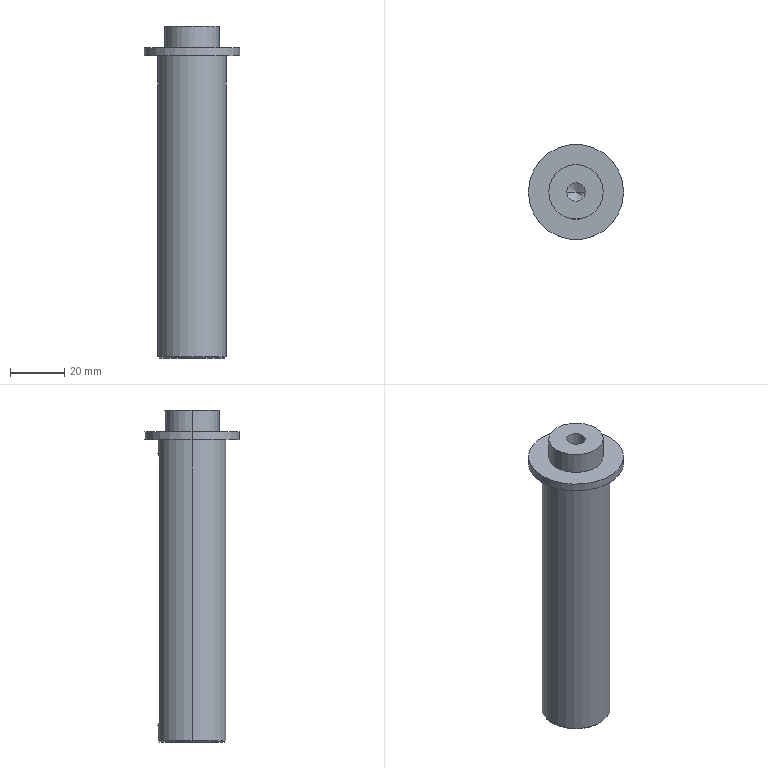Part | SolidWorks | features ICE 3, HoleWzd 2, Chamfer 1, Extrusion 1 | 1 solid | 26 faces | box 35 x 35 x 122 mm | volume 53457 mm3 | cylinder 13 | plane 7 | cone 6 | commonest cylinder face diameters 8 x3 6.8 x2 10.2 x2 20 x2 25 x2 35 x2
STEP:
#1=CARTESIAN_POINT('',(-12.,0.,0.));
#2=VERTEX_POINT('',#1);
#3=CARTESIAN_POINT('',(12.,0.,0.));
#4=VERTEX_POINT('',#3);
#5=CARTESIAN_POINT('',(0.,0.,0.));
#6=DIRECTION('',(0.,0.,-1.));
#7=DIRECTION('',(1.,0.,0.));
#8=AXIS2_PLACEMENT_3D('',#5,#6,#7);
#9=CIRCLE('',#8,12.);
#10=EDGE_CURVE('',#2,#4,#9,.T.);
#11=ORIENTED_EDGE('',*,*,#10,.F.);
#12=CARTESIAN_POINT('',(-12.5,0.,0.5));
#13=VERTEX_POINT('',#12);
#14=CARTESIAN_POINT('',(-12.5,0.,0.5));
#15=DIRECTION('',(-0.7071,0.,0.7071));
#16=VECTOR('',#15,1000.);
#17=LINE('',#14,#16);
#18=EDGE_CURVE('',#2,#13,#17,.T.);
#19=ORIENTED_EDGE('',*,*,#18,.T.);
#20=CARTESIAN_POINT('',(12.5,0.,0.5));
#21=VERTEX_POINT('',#20);
#22=CARTESIAN_POINT('',(0.,0.,0.5));
#23=DIRECTION('',(0.,0.,1.));
#24=DIRECTION('',(1.,0.,0.));
#25=AXIS2_PLACEMENT_3D('',#22,#23,#24);
#26=CIRCLE('',#25,12.5);
#27=EDGE_CURVE('',#21,#13,#26,.T.);
#28=ORIENTED_EDGE('',*,*,#27,.F.);
#29=CARTESIAN_POINT('',(12.5,0.,0.5));
#30=DIRECTION('',(0.7071,0.,0.7071));
#31=VECTOR('',#30,1000.);
#32=LINE('',#29,#31);
#33=EDGE_CURVE('',#4,#21,#32,.T.);
#34=ORIENTED_EDGE('',*,*,#33,.F.);
#35=EDGE_LOOP('',(#11,#19,#28,#34));
#36=FACE_OUTER_BOUND('',#35,.T.);
#37=CARTESIAN_POINT('',(0.,0.,0.5));
#38=DIRECTION('',(0.,0.,1.));
#39=DIRECTION('',(1.,0.,0.));
#40=AXIS2_PLACEMENT_3D('',#37,#38,#39);
#41=CONICAL_SURFACE('',#40,12.5,0.7854);
#42=ADVANCED_FACE('',(#36),#41,.T.);
#43=CARTESIAN_POINT('',(5.1,0.,30.25));
#44=VERTEX_POINT('',#43);
#45=CARTESIAN_POINT('',(-5.1,0.,30.25));
#46=VERTEX_POINT('',#45);
#47=CARTESIAN_POINT('',(0.,0.,30.25));
#48=DIRECTION('',(0.,0.,-1.));
#49=DIRECTION('',(-1.,0.,0.));
#50=AXIS2_PLACEMENT_3D('',#47,#48,#49);
#51=CIRCLE('',#50,5.1);
#52=EDGE_CURVE('',#44,#46,#51,.T.);
#53=ORIENTED_EDGE('',*,*,#52,.F.);
#54=CARTESIAN_POINT('',(5.1,0.,0.));
#55=VERTEX_POINT('',#54);
#56=CARTESIAN_POINT('',(5.1,0.,0.));
#57=DIRECTION('',(0.,0.,-1.));
#58=VECTOR('',#57,1000.);
#59=LINE('',#56,#58);
#60=EDGE_CURVE('',#44,#55,#59,.T.);
#61=ORIENTED_EDGE('',*,*,#60,.T.);
#62=CARTESIAN_POINT('',(-5.1,0.,0.));
#63=VERTEX_POINT('',#62);
#64=CARTESIAN_POINT('',(0.,0.,0.));
#65=DIRECTION('',(0.,0.,-1.));
#66=DIRECTION('',(-1.,0.,0.));
#67=AXIS2_PLACEMENT_3D('',#64,#65,#66);
#68=CIRCLE('',#67,5.1);
#69=EDGE_CURVE('',#55,#63,#68,.T.);
#70=ORIENTED_EDGE('',*,*,#69,.T.);
#71=CARTESIAN_POINT('',(-5.1,0.,0.));
#72=DIRECTION('',(0.,0.,-1.));
#73=VECTOR('',#72,1000.);
#74=LINE('',#71,#73);
#75=EDGE_CURVE('',#46,#63,#74,.T.);
#76=ORIENTED_EDGE('',*,*,#75,.F.);
#77=EDGE_LOOP('',(#53,#61,#70,#76));
#78=FACE_OUTER_BOUND('',#77,.T.);
#79=CARTESIAN_POINT('',(0.,0.,0.));
#80=DIRECTION('',(0.,0.,-1.));
#81=DIRECTION('',(-1.,0.,0.));
#82=AXIS2_PLACEMENT_3D('',#79,#80,#81);
#83=CYLINDRICAL_SURFACE('',#82,5.1);
#84=ADVANCED_FACE('',(#78),#83,.F.);
#85=CARTESIAN_POINT('',(0.,0.,33.314));
#86=VERTEX_POINT('',#85);
#87=CARTESIAN_POINT('',(-5.1,0.,30.25));
#88=DIRECTION('',(-0.8572,0.,-0.515));
#89=VECTOR('',#88,1000.);
#90=LINE('',#87,#89);
#91=EDGE_CURVE('',#86,#46,#90,.T.);
#92=ORIENTED_EDGE('',*,*,#91,.F.);
#93=CARTESIAN_POINT('',(5.1,0.,30.25));
#94=DIRECTION('',(0.8572,0.,-0.515));
#95=VECTOR('',#94,1000.);
#96=LINE('',#93,#95);
#97=EDGE_CURVE('',#86,#44,#96,.T.);
#98=ORIENTED_EDGE('',*,*,#97,.T.);
#99=ORIENTED_EDGE('',*,*,#52,.T.);
#100=EDGE_LOOP('',(#92,#98,#99));
#101=FACE_OUTER_BOUND('',#100,.T.);
#102=CARTESIAN_POINT('',(0.,0.,30.25));
#103=DIRECTION('',(0.,0.,-1.));
#104=DIRECTION('',(-1.,0.,0.));
#105=AXIS2_PLACEMENT_3D('',#102,#103,#104);
#106=CONICAL_SURFACE('',#105,5.1,1.03);
#107=ADVANCED_FACE('',(#101),#106,.F.);
#108=CARTESIAN_POINT('',(-3.4,0.,98.25));
#109=VERTEX_POINT('',#108);
#110=CARTESIAN_POINT('',(3.4,0.,98.25));
#111=VERTEX_POINT('',#110);
#112=CARTESIAN_POINT('',(0.,0.,98.25));
#113=DIRECTION('',(0.,0.,1.));
#114=DIRECTION('',(1.,0.,0.));
#115=AXIS2_PLACEMENT_3D('',#112,#113,#114);
#116=CIRCLE('',#115,3.4);
#117=EDGE_CURVE('',#109,#111,#116,.T.);
#118=ORIENTED_EDGE('',*,*,#117,.F.);
#119=CARTESIAN_POINT('',(-3.4,0.,122.));
#120=VERTEX_POINT('',#119);
#121=CARTESIAN_POINT('',(-3.4,0.,122.));
#122=DIRECTION('',(0.,0.,1.));
#123=VECTOR('',#122,1000.);
#124=LINE('',#121,#123);
#125=EDGE_CURVE('',#109,#120,#124,.T.);
#126=ORIENTED_EDGE('',*,*,#125,.T.);
#127=CARTESIAN_POINT('',(3.4,0.,122.));
#128=VERTEX_POINT('',#127);
#129=CARTESIAN_POINT('',(0.,0.,122.));
#130=DIRECTION('',(0.,0.,1.));
#131=DIRECTION('',(1.,0.,0.));
#132=AXIS2_PLACEMENT_3D('',#129,#130,#131);
#133=CIRCLE('',#132,3.4);
#134=EDGE_CURVE('',#120,#128,#133,.T.);
#135=ORIENTED_EDGE('',*,*,#134,.T.);
#136=CARTESIAN_POINT('',(3.4,0.,122.));
#137=DIRECTION('',(0.,0.,1.));
#138=VECTOR('',#137,1000.);
#139=LINE('',#136,#138);
#140=EDGE_CURVE('',#111,#128,#139,.T.);
#141=ORIENTED_EDGE('',*,*,#140,.F.);
#142=EDGE_LOOP('',(#118,#126,#135,#141));
#143=FACE_OUTER_BOUND('',#142,.T.);
#144=CARTESIAN_POINT('',(0.,0.,122.));
#145=DIRECTION('',(0.,0.,1.));
#146=DIRECTION('',(1.,0.,0.));
#147=AXIS2_PLACEMENT_3D('',#144,#145,#146);
#148=CYLINDRICAL_SURFACE('',#147,3.4);
#149=ADVANCED_FACE('',(#143),#148,.F.);
#150=CARTESIAN_POINT('',(0.,0.,96.207));
#151=VERTEX_POINT('',#150);
#152=CARTESIAN_POINT('',(3.4,0.,98.25));
#153=DIRECTION('',(0.8572,0.,0.515));
#154=VECTOR('',#153,1000.);
#155=LINE('',#152,#154);
#156=EDGE_CURVE('',#151,#111,#155,.T.);
#157=ORIENTED_EDGE('',*,*,#156,.F.);
#158=CARTESIAN_POINT('',(-3.4,0.,98.25));
#159=DIRECTION('',(-0.8572,0.,0.515));
#160=VECTOR('',#159,1000.);
#161=LINE('',#158,#160);
#162=EDGE_CURVE('',#151,#109,#161,.T.);
#163=ORIENTED_EDGE('',*,*,#162,.T.);
#164=ORIENTED_EDGE('',*,*,#117,.T.);
#165=EDGE_LOOP('',(#157,#163,#164));
#166=FACE_OUTER_BOUND('',#165,.T.);
#167=CARTESIAN_POINT('',(0.,0.,98.25));
#168=DIRECTION('',(0.,0.,1.));
#169=DIRECTION('',(1.,0.,0.));
#170=AXIS2_PLACEMENT_3D('',#167,#168,#169);
#171=CONICAL_SURFACE('',#170,3.4,1.03);
#172=ADVANCED_FACE('',(#166),#171,.F.);
#173=CARTESIAN_POINT('',(0.,8.5,106.));
#174=VERTEX_POINT('',#173);
#175=CARTESIAN_POINT('',(4.,8.5,102.));
#176=VERTEX_POINT('',#175);
#177=CARTESIAN_POINT('',(0.,8.5,102.));
#178=DIRECTION('',(0.,1.,0.));
#179=DIRECTION('',(0.,0.,1.));
#180=AXIS2_PLACEMENT_3D('',#177,#178,#179);
#181=CIRCLE('',#180,4.);
#182=EDGE_CURVE('',#174,#176,#181,.T.);
#183=ORIENTED_EDGE('',*,*,#182,.F.);
#184=CARTESIAN_POINT('',(0.,12.5,106.));
#185=VERTEX_POINT('',#184);
#186=CARTESIAN_POINT('',(0.,8.5,106.));
#187=DIRECTION('',(0.,1.,0.));
#188=VECTOR('',#187,1000.);
#189=LINE('',#186,#188);
#190=EDGE_CURVE('',#174,#185,#189,.T.);
#191=ORIENTED_EDGE('',*,*,#190,.T.);
#192=CARTESIAN_POINT('',(4.,11.843,102.));
#193=VERTEX_POINT('',#192);
#194=CARTESIAN_POINT('',(4.,11.843,102.));
#195=CARTESIAN_POINT('',(4.,11.843,102.266));
#196=CARTESIAN_POINT('',(3.974,11.852,102.528));
#197=CARTESIAN_POINT('',(3.871,11.886,103.041));
#198=CARTESIAN_POINT('',(3.793,11.911,103.296));
#199=CARTESIAN_POINT('',(3.592,11.973,103.78));
#200=CARTESIAN_POINT('',(3.469,12.01,104.009));
#201=CARTESIAN_POINT('',(3.178,12.09,104.443));
#202=CARTESIAN_POINT('',(3.011,12.134,104.646));
#203=CARTESIAN_POINT('',(2.644,12.219,105.013));
#204=CARTESIAN_POINT('',(2.444,12.261,105.178));
#205=CARTESIAN_POINT('',(2.006,12.34,105.47));
#206=CARTESIAN_POINT('',(1.776,12.375,105.593));
#207=CARTESIAN_POINT('',(1.295,12.435,105.793));
#208=CARTESIAN_POINT('',(1.041,12.459,105.871));
#209=CARTESIAN_POINT('',(0.5239,12.492,105.974));
#210=CARTESIAN_POINT('',(0.263,12.5,106.));
#211=CARTESIAN_POINT('',(0.,12.5,106.));
#212=B_SPLINE_CURVE_WITH_KNOTS('',3,(#194,#195,#196,#197,#198,#199,#200,#201,#202,#203,#204,#205,#206,#207,#208,#209,#210,#211),.UNSPECIFIED.,.F.,.F.,(4,2,2,2,2,2,2,2,4),(0.,0.000787,0.001574,0.002361,0.003148,0.003935,0.004722,0.005509,0.006296),.UNSPECIFIED.);
#213=EDGE_CURVE('',#193,#185,#212,.T.);
#214=ORIENTED_EDGE('',*,*,#213,.F.);
#215=CARTESIAN_POINT('',(4.,8.5,102.));
#216=DIRECTION('',(0.,1.,0.));
#217=VECTOR('',#216,1000.);
#218=LINE('',#215,#217);
#219=EDGE_CURVE('',#176,#193,#218,.T.);
#220=ORIENTED_EDGE('',*,*,#219,.F.);
#221=EDGE_LOOP('',(#183,#191,#214,#220));
#222=FACE_OUTER_BOUND('',#221,.T.);
#223=CARTESIAN_POINT('',(0.,8.5,102.));
#224=DIRECTION('',(0.,1.,0.));
#225=DIRECTION('',(0.,0.,1.));
#226=AXIS2_PLACEMENT_3D('',#223,#224,#225);
#227=CYLINDRICAL_SURFACE('',#226,4.);
#228=ADVANCED_FACE('',(#222),#227,.F.);
#229=CARTESIAN_POINT('',(10.,0.,122.));
#230=VERTEX_POINT('',#229);
#231=CARTESIAN_POINT('',(-10.,0.,122.));
#232=VERTEX_POINT('',#231);
#233=CARTESIAN_POINT('',(0.,0.,122.));
#234=DIRECTION('',(0.,0.,1.));
#235=DIRECTION('',(1.,0.,0.));
#236=AXIS2_PLACEMENT_3D('',#233,#234,#235);
#237=CIRCLE('',#236,10.);
#238=EDGE_CURVE('',#230,#232,#237,.T.);
#239=ORIENTED_EDGE('',*,*,#238,.F.);
#240=CARTESIAN_POINT('',(10.,0.,114.));
#241=VERTEX_POINT('',#240);
#242=CARTESIAN_POINT('',(10.,0.,122.));
#243=DIRECTION('',(0.,0.,-1.));
#244=VECTOR('',#243,1000.);
#245=LINE('',#242,#244);
#246=EDGE_CURVE('',#230,#241,#245,.T.);
#247=ORIENTED_EDGE('',*,*,#246,.T.);
#248=CARTESIAN_POINT('',(-10.,0.,114.));
#249=VERTEX_POINT('',#248);
#250=CARTESIAN_POINT('',(0.,0.,114.));
#251=DIRECTION('',(0.,0.,1.));
#252=DIRECTION('',(1.,0.,0.));
#253=AXIS2_PLACEMENT_3D('',#250,#251,#252);
#254=CIRCLE('',#253,10.);
#255=EDGE_CURVE('',#241,#249,#254,.T.);
#256=ORIENTED_EDGE('',*,*,#255,.T.);
#257=CARTESIAN_POINT('',(-10.,0.,122.));
#258=DIRECTION('',(0.,0.,-1.));
#259=VECTOR('',#258,1000.);
#260=LINE('',#257,#259);
#261=EDGE_CURVE('',#232,#249,#260,.T.);
#262=ORIENTED_EDGE('',*,*,#261,.F.);
#263=EDGE_LOOP('',(#239,#247,#256,#262));
#264=FACE_OUTER_BOUND('',#263,.T.);
#265=CARTESIAN_POINT('',(0.,0.,122.));
#266=DIRECTION('',(0.,0.,-1.));
#267=DIRECTION('',(-1.,0.,0.));
#268=AXIS2_PLACEMENT_3D('',#265,#266,#267);
#269=CYLINDRICAL_SURFACE('',#268,10.);
#270=ADVANCED_FACE('',(#264),#269,.T.);
#271=CARTESIAN_POINT('',(17.5,0.,114.));
#272=VERTEX_POINT('',#271);
#273=CARTESIAN_POINT('',(-17.5,0.,114.));
#274=VERTEX_POINT('',#273);
#275=CARTESIAN_POINT('',(0.,0.,114.));
#276=DIRECTION('',(0.,0.,1.));
#277=DIRECTION('',(1.,0.,0.));
#278=AXIS2_PLACEMENT_3D('',#275,#276,#277);
#279=CIRCLE('',#278,17.5);
#280=EDGE_CURVE('',#272,#274,#279,.T.);
#281=ORIENTED_EDGE('',*,*,#280,.F.);
#282=CARTESIAN_POINT('',(17.5,0.,111.));
#283=VERTEX_POINT('',#282);
#284=CARTESIAN_POINT('',(17.5,0.,114.));
#285=DIRECTION('',(0.,0.,-1.));
#286=VECTOR('',#285,1000.);
#287=LINE('',#284,#286);
#288=EDGE_CURVE('',#272,#283,#287,.T.);
#289=ORIENTED_EDGE('',*,*,#288,.T.);
#290=CARTESIAN_POINT('',(-17.5,0.,111.));
#291=VERTEX_POINT('',#290);
#292=CARTESIAN_POINT('',(0.,0.,111.));
#293=DIRECTION('',(0.,0.,1.));
#294=DIRECTION('',(1.,0.,0.));
#295=AXIS2_PLACEMENT_3D('',#292,#293,#294);
#296=CIRCLE('',#295,17.5);
#297=EDGE_CURVE('',#283,#291,#296,.T.);
#298=ORIENTED_EDGE('',*,*,#297,.T.);
#299=CARTESIAN_POINT('',(-17.5,0.,114.));
#300=DIRECTION('',(0.,0.,-1.));
#301=VECTOR('',#300,1000.);
#302=LINE('',#299,#301);
#303=EDGE_CURVE('',#274,#291,#302,.T.);
#304=ORIENTED_EDGE('',*,*,#303,.F.);
#305=EDGE_LOOP('',(#281,#289,#298,#304));
#306=FACE_OUTER_BOUND('',#305,.T.);
#307=CARTESIAN_POINT('',(0.,0.,114.));
#308=DIRECTION('',(0.,0.,-1.));
#309=DIRECTION('',(-1.,0.,0.));
#310=AXIS2_PLACEMENT_3D('',#307,#308,#309);
#311=CYLINDRICAL_SURFACE('',#310,17.5);
#312=ADVANCED_FACE('',(#306),#311,.T.);
#313=CARTESIAN_POINT('',(4.,11.843,10.));
#314=VERTEX_POINT('',#313);
#315=CARTESIAN_POINT('',(4.,11.843,111.));
#316=DIRECTION('',(0.,0.,1.));
#317=VECTOR('',#316,1000.);
#318=LINE('',#315,#317);
#319=EDGE_CURVE('',#314,#193,#318,.T.);
#320=ORIENTED_EDGE('',*,*,#319,.T.);
#321=ORIENTED_EDGE('',*,*,#213,.T.);
#322=CARTESIAN_POINT('',(-4.,11.843,102.));
#323=VERTEX_POINT('',#322);
#324=CARTESIAN_POINT('',(0.,12.5,106.));
#325=CARTESIAN_POINT('',(-0.2627,12.5,106.));
#326=CARTESIAN_POINT('',(-0.5294,12.491,105.973));
#327=CARTESIAN_POINT('',(-1.043,12.459,105.87));
#328=CARTESIAN_POINT('',(-1.293,12.435,105.794));
#329=CARTESIAN_POINT('',(-1.78,12.375,105.592));
#330=CARTESIAN_POINT('',(-2.011,12.339,105.468));
#331=CARTESIAN_POINT('',(-2.442,12.261,105.179));
#332=CARTESIAN_POINT('',(-2.645,12.218,105.012));
#333=CARTESIAN_POINT('',(-3.013,12.133,104.644));
#334=CARTESIAN_POINT('',(-3.177,12.09,104.444));
#335=CARTESIAN_POINT('',(-3.467,12.011,104.012));
#336=CARTESIAN_POINT('',(-3.592,11.973,103.778));
#337=CARTESIAN_POINT('',(-3.793,11.911,103.297));
#338=CARTESIAN_POINT('',(-3.869,11.886,103.048));
#339=CARTESIAN_POINT('',(-3.973,11.852,102.532));
#340=CARTESIAN_POINT('',(-4.,11.843,102.266));
#341=CARTESIAN_POINT('',(-4.,11.843,102.));
#342=B_SPLINE_CURVE_WITH_KNOTS('',3,(#324,#325,#326,#327,#328,#329,#330,#331,#332,#333,#334,#335,#336,#337,#338,#339,#340,#341),.UNSPECIFIED.,.F.,.F.,(4,2,2,2,2,2,2,2,4),(0.006296,0.007082,0.007868,0.008654,0.00944,0.01023,0.01101,0.0118,0.01258),.UNSPECIFIED.);
#343=EDGE_CURVE('',#185,#323,#342,.T.);
#344=ORIENTED_EDGE('',*,*,#343,.T.);
#345=CARTESIAN_POINT('',(-4.,11.843,10.));
#346=VERTEX_POINT('',#345);
#347=CARTESIAN_POINT('',(-4.,11.843,111.));
#348=DIRECTION('',(0.,0.,-1.));
#349=VECTOR('',#348,1000.);
#350=LINE('',#347,#349);
#351=EDGE_CURVE('',#323,#346,#350,.T.);
#352=ORIENTED_EDGE('',*,*,#351,.T.);
#353=CARTESIAN_POINT('',(-4.,11.843,10.));
#354=CARTESIAN_POINT('',(-4.,11.843,9.734));
#355=CARTESIAN_POINT('',(-3.974,11.852,9.473));
#356=CARTESIAN_POINT('',(-3.871,11.886,8.959));
#357=CARTESIAN_POINT('',(-3.793,11.911,8.704));
#358=CARTESIAN_POINT('',(-3.592,11.973,8.221));
#359=CARTESIAN_POINT('',(-3.469,12.01,7.992));
#360=CARTESIAN_POINT('',(-3.179,12.09,7.559));
#361=CARTESIAN_POINT('',(-3.012,12.133,7.355));
#362=CARTESIAN_POINT('',(-2.646,12.218,6.989));
#363=CARTESIAN_POINT('',(-2.445,12.26,6.824));
#364=CARTESIAN_POINT('',(-2.009,12.34,6.531));
#365=CARTESIAN_POINT('',(-1.779,12.375,6.408));
#366=CARTESIAN_POINT('',(-1.299,12.435,6.208));
#367=CARTESIAN_POINT('',(-1.045,12.459,6.13));
#368=CARTESIAN_POINT('',(-0.5276,12.492,6.026));
#369=CARTESIAN_POINT('',(-0.2669,12.5,6.));
#370=CARTESIAN_POINT('',(0.2587,12.5,6.));
#371=CARTESIAN_POINT('',(0.5256,12.492,6.026));
#372=CARTESIAN_POINT('',(1.04,12.459,6.129));
#373=CARTESIAN_POINT('',(1.29,12.436,6.205));
#374=CARTESIAN_POINT('',(1.777,12.375,6.407));
#375=CARTESIAN_POINT('',(2.008,12.34,6.531));
#376=CARTESIAN_POINT('',(2.44,12.262,6.82));
#377=CARTESIAN_POINT('',(2.643,12.219,6.987));
#378=CARTESIAN_POINT('',(3.012,12.133,7.355));
#379=CARTESIAN_POINT('',(3.176,12.091,7.555));
#380=CARTESIAN_POINT('',(3.466,12.011,7.987));
#381=CARTESIAN_POINT('',(3.592,11.973,8.22));
#382=CARTESIAN_POINT('',(3.792,11.911,8.702));
#383=CARTESIAN_POINT('',(3.869,11.886,8.951));
#384=CARTESIAN_POINT('',(3.973,11.852,9.468));
#385=CARTESIAN_POINT('',(4.,11.843,9.734));
#386=CARTESIAN_POINT('',(4.,11.843,10.));
#387=B_SPLINE_CURVE_WITH_KNOTS('',3,(#353,#354,#355,#356,#357,#358,#359,#360,#361,#362,#363,#364,#365,#366,#367,#368,#369,#370,#371,#372,#373,#374,#375,#376,#377,#378,#379,#380,#381,#382,#383,#384,#385,#386),.UNSPECIFIED.,.F.,.F.,(4,2,2,2,2,2,2,2,2,2,2,2,2,2,2,2,4),(0.,0.0007865,0.001573,0.00236,0.003146,0.003933,0.004719,0.005506,0.006292,0.007079,0.007865,0.008652,0.009438,0.01022,0.01101,0.0118,0.01258),.UNSPECIFIED.);
#388=EDGE_CURVE('',#346,#314,#387,.T.);
#389=ORIENTED_EDGE('',*,*,#388,.T.);
#390=EDGE_LOOP('',(#320,#321,#344,#352,#389));
#391=FACE_BOUND('',#390,.T.);
#392=CARTESIAN_POINT('',(12.5,0.,111.));
#393=VERTEX_POINT('',#392);
#394=CARTESIAN_POINT('',(-12.5,0.,111.));
#395=VERTEX_POINT('',#394);
#396=CARTESIAN_POINT('',(0.,0.,111.));
#397=DIRECTION('',(0.,0.,1.));
#398=DIRECTION('',(1.,0.,0.));
#399=AXIS2_PLACEMENT_3D('',#396,#397,#398);
#400=CIRCLE('',#399,12.5);
#401=EDGE_CURVE('',#393,#395,#400,.T.);
#402=ORIENTED_EDGE('',*,*,#401,.F.);
#403=CARTESIAN_POINT('',(12.5,0.,111.));
#404=DIRECTION('',(0.,0.,-1.));
#405=VECTOR('',#404,1000.);
#406=LINE('',#403,#405);
#407=EDGE_CURVE('',#393,#21,#406,.T.);
#408=ORIENTED_EDGE('',*,*,#407,.T.);
#409=ORIENTED_EDGE('',*,*,#27,.T.);
#410=CARTESIAN_POINT('',(-12.5,0.,111.));
#411=DIRECTION('',(0.,0.,-1.));
#412=VECTOR('',#411,1000.);
#413=LINE('',#410,#412);
#414=EDGE_CURVE('',#395,#13,#413,.T.);
#415=ORIENTED_EDGE('',*,*,#414,.F.);
#416=EDGE_LOOP('',(#402,#408,#409,#415));
#417=FACE_OUTER_BOUND('',#416,.T.);
#418=CARTESIAN_POINT('',(0.,0.,111.));
#419=DIRECTION('',(0.,0.,-1.));
#420=DIRECTION('',(-1.,0.,0.));
#421=AXIS2_PLACEMENT_3D('',#418,#419,#420);
#422=CYLINDRICAL_SURFACE('',#421,12.5);
#423=ADVANCED_FACE('',(#391,#417),#422,.T.);
#424=ORIENTED_EDGE('',*,*,#407,.F.);
#425=CARTESIAN_POINT('',(0.,0.,111.));
#426=DIRECTION('',(0.,0.,1.));
#427=DIRECTION('',(1.,0.,0.));
#428=AXIS2_PLACEMENT_3D('',#425,#426,#427);
#429=CIRCLE('',#428,12.5);
#430=EDGE_CURVE('',#395,#393,#429,.T.);
#431=ORIENTED_EDGE('',*,*,#430,.F.);
#432=ORIENTED_EDGE('',*,*,#414,.T.);
#433=CARTESIAN_POINT('',(0.,0.,0.5));
#434=DIRECTION('',(0.,0.,1.));
#435=DIRECTION('',(1.,0.,0.));
#436=AXIS2_PLACEMENT_3D('',#433,#434,#435);
#437=CIRCLE('',#436,12.5);
#438=EDGE_CURVE('',#13,#21,#437,.T.);
#439=ORIENTED_EDGE('',*,*,#438,.T.);
#440=EDGE_LOOP('',(#424,#431,#432,#439));
#441=FACE_OUTER_BOUND('',#440,.T.);
#442=CARTESIAN_POINT('',(0.,0.,111.));
#443=DIRECTION('',(0.,0.,-1.));
#444=DIRECTION('',(-1.,0.,0.));
#445=AXIS2_PLACEMENT_3D('',#442,#443,#444);
#446=CYLINDRICAL_SURFACE('',#445,12.5);
#447=ADVANCED_FACE('',(#441),#446,.T.);
#448=CARTESIAN_POINT('',(0.,0.,0.));
#449=DIRECTION('',(0.,0.,-1.));
#450=DIRECTION('',(1.,0.,0.));
#451=AXIS2_PLACEMENT_3D('',#448,#449,#450);
#452=CIRCLE('',#451,12.);
#453=EDGE_CURVE('',#4,#2,#452,.T.);
#454=ORIENTED_EDGE('',*,*,#453,.T.);
#455=ORIENTED_EDGE('',*,*,#10,.T.);
#456=EDGE_LOOP('',(#454,#455));
#457=FACE_OUTER_BOUND('',#456,.T.);
#458=CARTESIAN_POINT('',(0.,0.,0.));
#459=DIRECTION('',(0.,0.,-1.));
#460=DIRECTION('',(-1.,0.,0.));
#461=AXIS2_PLACEMENT_3D('',#458,#459,#460);
#462=CIRCLE('',#461,5.1);
#463=EDGE_CURVE('',#63,#55,#462,.T.);
#464=ORIENTED_EDGE('',*,*,#463,.F.);
#465=ORIENTED_EDGE('',*,*,#69,.F.);
#466=EDGE_LOOP('',(#464,#465));
#467=FACE_BOUND('',#466,.T.);
#468=CARTESIAN_POINT('',(0.,0.,0.));
#469=DIRECTION('',(0.,0.,1.));
#470=DIRECTION('',(1.,0.,0.));
#471=AXIS2_PLACEMENT_3D('',#468,#469,#470);
#472=PLANE('',#471);
#473=ADVANCED_FACE('',(#457,#467),#472,.F.);
#474=ORIENTED_EDGE('',*,*,#288,.F.);
#475=CARTESIAN_POINT('',(0.,0.,114.));
#476=DIRECTION('',(0.,0.,1.));
#477=DIRECTION('',(1.,0.,0.));
#478=AXIS2_PLACEMENT_3D('',#475,#476,#477);
#479=CIRCLE('',#478,17.5);
#480=EDGE_CURVE('',#274,#272,#479,.T.);
#481=ORIENTED_EDGE('',*,*,#480,.F.);
#482=ORIENTED_EDGE('',*,*,#303,.T.);
#483=CARTESIAN_POINT('',(0.,0.,111.));
#484=DIRECTION('',(0.,0.,1.));
#485=DIRECTION('',(1.,0.,0.));
#486=AXIS2_PLACEMENT_3D('',#483,#484,#485);
#487=CIRCLE('',#486,17.5);
#488=EDGE_CURVE('',#291,#283,#487,.T.);
#489=ORIENTED_EDGE('',*,*,#488,.T.);
#490=EDGE_LOOP('',(#474,#481,#482,#489));
#491=FACE_OUTER_BOUND('',#490,.T.);
#492=CARTESIAN_POINT('',(0.,0.,114.));
#493=DIRECTION('',(0.,0.,-1.));
#494=DIRECTION('',(-1.,0.,0.));
#495=AXIS2_PLACEMENT_3D('',#492,#493,#494);
#496=CYLINDRICAL_SURFACE('',#495,17.5);
#497=ADVANCED_FACE('',(#491),#496,.T.);
#498=CARTESIAN_POINT('',(0.,0.,114.));
#499=DIRECTION('',(0.,0.,1.));
#500=DIRECTION('',(1.,0.,0.));
#501=AXIS2_PLACEMENT_3D('',#498,#499,#500);
#502=CIRCLE('',#501,10.);
#503=EDGE_CURVE('',#249,#241,#502,.T.);
#504=ORIENTED_EDGE('',*,*,#503,.F.);
#505=ORIENTED_EDGE('',*,*,#255,.F.);
#506=EDGE_LOOP('',(#504,#505));
#507=FACE_BOUND('',#506,.T.);
#508=ORIENTED_EDGE('',*,*,#480,.T.);
#509=ORIENTED_EDGE('',*,*,#280,.T.);
#510=EDGE_LOOP('',(#508,#509));
#511=FACE_OUTER_BOUND('',#510,.T.);
#512=CARTESIAN_POINT('',(0.,0.,114.));
#513=DIRECTION('',(0.,0.,1.));
#514=DIRECTION('',(1.,0.,0.));
#515=AXIS2_PLACEMENT_3D('',#512,#513,#514);
#516=PLANE('',#515);
#517=ADVANCED_FACE('',(#507,#511),#516,.T.);
#518=ORIENTED_EDGE('',*,*,#430,.T.);
#519=ORIENTED_EDGE('',*,*,#401,.T.);
#520=EDGE_LOOP('',(#518,#519));
#521=FACE_BOUND('',#520,.T.);
#522=ORIENTED_EDGE('',*,*,#488,.F.);
#523=ORIENTED_EDGE('',*,*,#297,.F.);
#524=EDGE_LOOP('',(#522,#523));
#525=FACE_OUTER_BOUND('',#524,.T.);
#526=CARTESIAN_POINT('',(0.,0.,111.));
#527=DIRECTION('',(0.,0.,1.));
#528=DIRECTION('',(1.,0.,0.));
#529=AXIS2_PLACEMENT_3D('',#526,#527,#528);
#530=PLANE('',#529);
#531=ADVANCED_FACE('',(#521,#525),#530,.F.);
#532=ORIENTED_EDGE('',*,*,#246,.F.);
#533=CARTESIAN_POINT('',(0.,0.,122.));
#534=DIRECTION('',(0.,0.,1.));
#535=DIRECTION('',(1.,0.,0.));
#536=AXIS2_PLACEMENT_3D('',#533,#534,#535);
#537=CIRCLE('',#536,10.);
#538=EDGE_CURVE('',#232,#230,#537,.T.);
#539=ORIENTED_EDGE('',*,*,#538,.F.);
#540=ORIENTED_EDGE('',*,*,#261,.T.);
#541=ORIENTED_EDGE('',*,*,#503,.T.);
#542=EDGE_LOOP('',(#532,#539,#540,#541));
#543=FACE_OUTER_BOUND('',#542,.T.);
#544=CARTESIAN_POINT('',(0.,0.,122.));
#545=DIRECTION('',(0.,0.,-1.));
#546=DIRECTION('',(-1.,0.,0.));
#547=AXIS2_PLACEMENT_3D('',#544,#545,#546);
#548=CYLINDRICAL_SURFACE('',#547,10.);
#549=ADVANCED_FACE('',(#543),#548,.T.);
#550=CARTESIAN_POINT('',(0.,0.,122.));
#551=DIRECTION('',(0.,0.,1.));
#552=DIRECTION('',(1.,0.,0.));
#553=AXIS2_PLACEMENT_3D('',#550,#551,#552);
#554=CIRCLE('',#553,3.4);
#555=EDGE_CURVE('',#128,#120,#554,.T.);
#556=ORIENTED_EDGE('',*,*,#555,.F.);
#557=ORIENTED_EDGE('',*,*,#134,.F.);
#558=EDGE_LOOP('',(#556,#557));
#559=FACE_BOUND('',#558,.T.);
#560=ORIENTED_EDGE('',*,*,#538,.T.);
#561=ORIENTED_EDGE('',*,*,#238,.T.);
#562=EDGE_LOOP('',(#560,#561));
#563=FACE_OUTER_BOUND('',#562,.T.);
#564=CARTESIAN_POINT('',(0.,0.,122.));
#565=DIRECTION('',(0.,0.,1.));
#566=DIRECTION('',(1.,0.,0.));
#567=AXIS2_PLACEMENT_3D('',#564,#565,#566);
#568=PLANE('',#567);
#569=ADVANCED_FACE('',(#559,#563),#568,.T.);
#570=CARTESIAN_POINT('',(-4.,8.5,10.));
#571=VERTEX_POINT('',#570);
#572=CARTESIAN_POINT('',(-4.,8.5,10.));
#573=DIRECTION('',(0.,1.,0.));
#574=VECTOR('',#573,1000.);
#575=LINE('',#572,#574);
#576=EDGE_CURVE('',#571,#346,#575,.T.);
#577=ORIENTED_EDGE('',*,*,#576,.F.);
#578=CARTESIAN_POINT('',(4.,8.5,10.));
#579=VERTEX_POINT('',#578);
#580=CARTESIAN_POINT('',(0.,8.5,10.));
#581=DIRECTION('',(0.,1.,0.));
#582=DIRECTION('',(0.,0.,1.));
#583=AXIS2_PLACEMENT_3D('',#580,#581,#582);
#584=CIRCLE('',#583,4.);
#585=EDGE_CURVE('',#579,#571,#584,.T.);
#586=ORIENTED_EDGE('',*,*,#585,.F.);
#587=CARTESIAN_POINT('',(4.,8.5,10.));
#588=DIRECTION('',(0.,1.,0.));
#589=VECTOR('',#588,1000.);
#590=LINE('',#587,#589);
#591=EDGE_CURVE('',#579,#314,#590,.T.);
#592=ORIENTED_EDGE('',*,*,#591,.T.);
#593=ORIENTED_EDGE('',*,*,#388,.F.);
#594=EDGE_LOOP('',(#577,#586,#592,#593));
#595=FACE_OUTER_BOUND('',#594,.T.);
#596=CARTESIAN_POINT('',(0.,8.5,10.));
#597=DIRECTION('',(0.,1.,0.));
#598=DIRECTION('',(0.,0.,1.));
#599=AXIS2_PLACEMENT_3D('',#596,#597,#598);
#600=CYLINDRICAL_SURFACE('',#599,4.);
#601=ADVANCED_FACE('',(#595),#600,.F.);
#602=ORIENTED_EDGE('',*,*,#591,.F.);
#603=CARTESIAN_POINT('',(4.,8.5,10.));
#604=DIRECTION('',(0.,0.,-1.));
#605=VECTOR('',#604,1000.);
#606=LINE('',#603,#605);
#607=EDGE_CURVE('',#176,#579,#606,.T.);
#608=ORIENTED_EDGE('',*,*,#607,.F.);
#609=ORIENTED_EDGE('',*,*,#219,.T.);
#610=ORIENTED_EDGE('',*,*,#319,.F.);
#611=EDGE_LOOP('',(#602,#608,#609,#610));
#612=FACE_OUTER_BOUND('',#611,.T.);
#613=CARTESIAN_POINT('',(4.,8.5,10.));
#614=DIRECTION('',(1.,0.,0.));
#615=DIRECTION('',(0.,0.,-1.));
#616=AXIS2_PLACEMENT_3D('',#613,#614,#615);
#617=PLANE('',#616);
#618=ADVANCED_FACE('',(#612),#617,.F.);
#619=ORIENTED_EDGE('',*,*,#190,.F.);
#620=CARTESIAN_POINT('',(-4.,8.5,102.));
#621=VERTEX_POINT('',#620);
#622=CARTESIAN_POINT('',(0.,8.5,102.));
#623=DIRECTION('',(0.,1.,0.));
#624=DIRECTION('',(0.,0.,1.));
#625=AXIS2_PLACEMENT_3D('',#622,#623,#624);
#626=CIRCLE('',#625,4.);
#627=EDGE_CURVE('',#621,#174,#626,.T.);
#628=ORIENTED_EDGE('',*,*,#627,.F.);
#629=CARTESIAN_POINT('',(-4.,8.5,102.));
#630=DIRECTION('',(0.,1.,0.));
#631=VECTOR('',#630,1000.);
#632=LINE('',#629,#631);
#633=EDGE_CURVE('',#621,#323,#632,.T.);
#634=ORIENTED_EDGE('',*,*,#633,.T.);
#635=ORIENTED_EDGE('',*,*,#343,.F.);
#636=EDGE_LOOP('',(#619,#628,#634,#635));
#637=FACE_OUTER_BOUND('',#636,.T.);
#638=CARTESIAN_POINT('',(0.,8.5,102.));
#639=DIRECTION('',(0.,1.,0.));
#640=DIRECTION('',(0.,0.,1.));
#641=AXIS2_PLACEMENT_3D('',#638,#639,#640);
#642=CYLINDRICAL_SURFACE('',#641,4.);
#643=ADVANCED_FACE('',(#637),#642,.F.);
#644=ORIENTED_EDGE('',*,*,#633,.F.);
#645=CARTESIAN_POINT('',(-4.,8.5,10.));
#646=DIRECTION('',(0.,0.,1.));
#647=VECTOR('',#646,1000.);
#648=LINE('',#645,#647);
#649=EDGE_CURVE('',#571,#621,#648,.T.);
#650=ORIENTED_EDGE('',*,*,#649,.F.);
#651=ORIENTED_EDGE('',*,*,#576,.T.);
#652=ORIENTED_EDGE('',*,*,#351,.F.);
#653=EDGE_LOOP('',(#644,#650,#651,#652));
#654=FACE_OUTER_BOUND('',#653,.T.);
#655=CARTESIAN_POINT('',(-4.,8.5,10.));
#656=DIRECTION('',(-1.,0.,0.));
#657=DIRECTION('',(0.,0.,1.));
#658=AXIS2_PLACEMENT_3D('',#655,#656,#657);
#659=PLANE('',#658);
#660=ADVANCED_FACE('',(#654),#659,.F.);
#661=ORIENTED_EDGE('',*,*,#585,.T.);
#662=ORIENTED_EDGE('',*,*,#649,.T.);
#663=ORIENTED_EDGE('',*,*,#627,.T.);
#664=ORIENTED_EDGE('',*,*,#182,.T.);
#665=ORIENTED_EDGE('',*,*,#607,.T.);
#666=EDGE_LOOP('',(#661,#662,#663,#664,#665));
#667=FACE_OUTER_BOUND('',#666,.T.);
#668=CARTESIAN_POINT('',(0.,8.5,10.));
#669=DIRECTION('',(0.,1.,0.));
#670=DIRECTION('',(0.,0.,1.));
#671=AXIS2_PLACEMENT_3D('',#668,#669,#670);
#672=PLANE('',#671);
#673=ADVANCED_FACE('',(#667),#672,.T.);
#674=ORIENTED_EDGE('',*,*,#162,.F.);
#675=ORIENTED_EDGE('',*,*,#156,.T.);
#676=CARTESIAN_POINT('',(0.,0.,98.25));
#677=DIRECTION('',(0.,0.,1.));
#678=DIRECTION('',(1.,0.,0.));
#679=AXIS2_PLACEMENT_3D('',#676,#677,#678);
#680=CIRCLE('',#679,3.4);
#681=EDGE_CURVE('',#111,#109,#680,.T.);
#682=ORIENTED_EDGE('',*,*,#681,.T.);
#683=EDGE_LOOP('',(#674,#675,#682));
#684=FACE_OUTER_BOUND('',#683,.T.);
#685=CARTESIAN_POINT('',(0.,0.,98.25));
#686=DIRECTION('',(0.,0.,1.));
#687=DIRECTION('',(1.,0.,0.));
#688=AXIS2_PLACEMENT_3D('',#685,#686,#687);
#689=CONICAL_SURFACE('',#688,3.4,1.03);
#690=ADVANCED_FACE('',(#684),#689,.F.);
#691=ORIENTED_EDGE('',*,*,#125,.F.);
#692=ORIENTED_EDGE('',*,*,#681,.F.);
#693=ORIENTED_EDGE('',*,*,#140,.T.);
#694=ORIENTED_EDGE('',*,*,#555,.T.);
#695=EDGE_LOOP('',(#691,#692,#693,#694));
#696=FACE_OUTER_BOUND('',#695,.T.);
#697=CARTESIAN_POINT('',(0.,0.,122.));
#698=DIRECTION('',(0.,0.,1.));
#699=DIRECTION('',(1.,0.,0.));
#700=AXIS2_PLACEMENT_3D('',#697,#698,#699);
#701=CYLINDRICAL_SURFACE('',#700,3.4);
#702=ADVANCED_FACE('',(#696),#701,.F.);
#703=ORIENTED_EDGE('',*,*,#97,.F.);
#704=ORIENTED_EDGE('',*,*,#91,.T.);
#705=CARTESIAN_POINT('',(0.,0.,30.25));
#706=DIRECTION('',(0.,0.,-1.));
#707=DIRECTION('',(-1.,0.,0.));
#708=AXIS2_PLACEMENT_3D('',#705,#706,#707);
#709=CIRCLE('',#708,5.1);
#710=EDGE_CURVE('',#46,#44,#709,.T.);
#711=ORIENTED_EDGE('',*,*,#710,.T.);
#712=EDGE_LOOP('',(#703,#704,#711));
#713=FACE_OUTER_BOUND('',#712,.T.);
#714=CARTESIAN_POINT('',(0.,0.,30.25));
#715=DIRECTION('',(0.,0.,-1.));
#716=DIRECTION('',(-1.,0.,0.));
#717=AXIS2_PLACEMENT_3D('',#714,#715,#716);
#718=CONICAL_SURFACE('',#717,5.1,1.03);
#719=ADVANCED_FACE('',(#713),#718,.F.);
#720=ORIENTED_EDGE('',*,*,#60,.F.);
#721=ORIENTED_EDGE('',*,*,#710,.F.);
#722=ORIENTED_EDGE('',*,*,#75,.T.);
#723=ORIENTED_EDGE('',*,*,#463,.T.);
#724=EDGE_LOOP('',(#720,#721,#722,#723));
#725=FACE_OUTER_BOUND('',#724,.T.);
#726=CARTESIAN_POINT('',(0.,0.,0.));
#727=DIRECTION('',(0.,0.,-1.));
#728=DIRECTION('',(-1.,0.,0.));
#729=AXIS2_PLACEMENT_3D('',#726,#727,#728);
#730=CYLINDRICAL_SURFACE('',#729,5.1);
#731=ADVANCED_FACE('',(#725),#730,.F.);
#732=ORIENTED_EDGE('',*,*,#18,.F.);
#733=ORIENTED_EDGE('',*,*,#453,.F.);
#734=ORIENTED_EDGE('',*,*,#33,.T.);
#735=ORIENTED_EDGE('',*,*,#438,.F.);
#736=EDGE_LOOP('',(#732,#733,#734,#735));
#737=FACE_OUTER_BOUND('',#736,.T.);
#738=CARTESIAN_POINT('',(0.,0.,0.5));
#739=DIRECTION('',(0.,0.,1.));
#740=DIRECTION('',(1.,0.,0.));
#741=AXIS2_PLACEMENT_3D('',#738,#739,#740);
#742=CONICAL_SURFACE('',#741,12.5,0.7854);
#743=ADVANCED_FACE('',(#737),#742,.T.);
#744=CLOSED_SHELL('',(#42,#84,#107,#149,#172,#228,#270,#312,#423,#447,#473,#497,#517,#531,#549,#569,#601,#618,#643,#660,#673,#690,#702,#719,#731,#743));
#745=MANIFOLD_SOLID_BREP('',#744);
#746=CARTESIAN_POINT('',(0.,0.,0.));
#747=DIRECTION('',(0.,0.,1.));
#748=DIRECTION('',(1.,0.,0.));
#749=AXIS2_PLACEMENT_3D('',#746,#747,#748);
#750=(LENGTH_UNIT()NAMED_UNIT(*)SI_UNIT(.MILLI.,.METRE.));
#751=UNCERTAINTY_MEASURE_WITH_UNIT(LENGTH_MEASURE(0.00001),#750,'','');
#752=(NAMED_UNIT(*)PLANE_ANGLE_UNIT()SI_UNIT($,.RADIAN.));
#753=(NAMED_UNIT(*)SI_UNIT($,.STERADIAN.)SOLID_ANGLE_UNIT());
#754=(GEOMETRIC_REPRESENTATION_CONTEXT(3)GLOBAL_UNCERTAINTY_ASSIGNED_CONTEXT((#751))GLOBAL_UNIT_ASSIGNED_CONTEXT((#750,#752,#753))REPRESENTATION_CONTEXT('',''));
#755=ADVANCED_BREP_SHAPE_REPRESENTATION('',(#745,#749),#754);